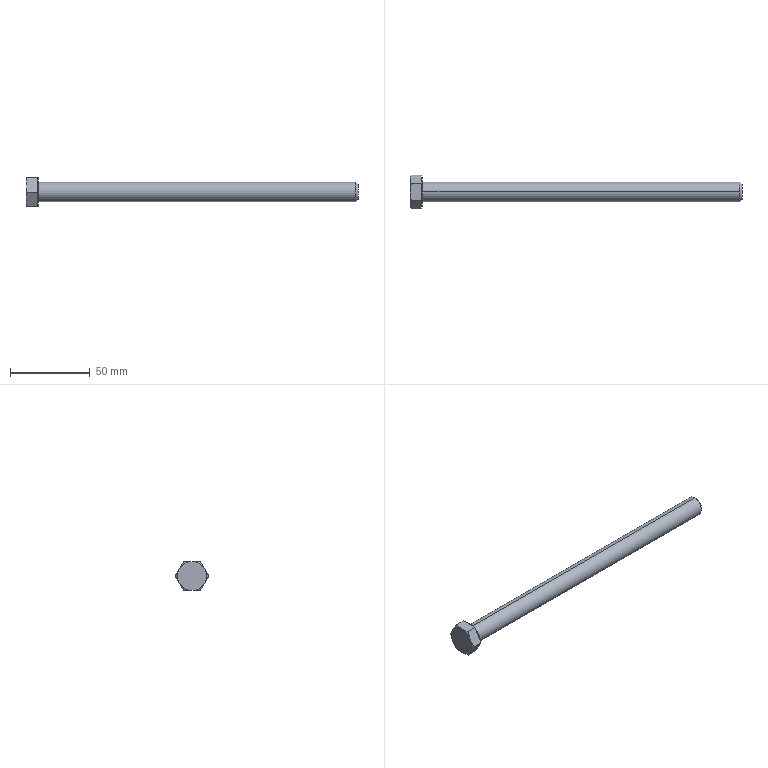Part | SolidWorks | features BaseBody 1 | 1 solid | 35 faces | box 207.5 x 20.785 x 18 mm | volume 24671 mm3 | plane 15 | cone 14 | cylinder 4 | torus 2 | commonest cylinder face diameters 12 x2 18 x2
STEP:
#1=CARTESIAN_POINT('',(8.1,0.,6.));
#2=VERTEX_POINT('',#1);
#3=CARTESIAN_POINT('',(7.5,0.,6.6));
#4=VERTEX_POINT('',#3);
#5=CARTESIAN_POINT('',(8.1,0.,6.6));
#6=DIRECTION('',(0.,1.,0.));
#7=DIRECTION('',(0.,0.,1.));
#8=AXIS2_PLACEMENT_3D('',#5,#6,#7);
#9=CIRCLE('',#8,0.6);
#10=EDGE_CURVE('',#2,#4,#9,.T.);
#11=ORIENTED_EDGE('',*,*,#10,.F.);
#12=CARTESIAN_POINT('',(8.1,0.,-6.));
#13=VERTEX_POINT('',#12);
#14=CARTESIAN_POINT('',(8.1,0.,0.));
#15=DIRECTION('',(1.,0.,0.));
#16=DIRECTION('',(0.,0.,-1.));
#17=AXIS2_PLACEMENT_3D('',#14,#15,#16);
#18=CIRCLE('',#17,6.);
#19=EDGE_CURVE('',#13,#2,#18,.T.);
#20=ORIENTED_EDGE('',*,*,#19,.F.);
#21=CARTESIAN_POINT('',(7.5,0.,-6.6));
#22=VERTEX_POINT('',#21);
#23=CARTESIAN_POINT('',(8.1,0.,-6.6));
#24=DIRECTION('',(0.,-1.,0.));
#25=DIRECTION('',(0.,0.,-1.));
#26=AXIS2_PLACEMENT_3D('',#23,#24,#25);
#27=CIRCLE('',#26,0.6);
#28=EDGE_CURVE('',#13,#22,#27,.T.);
#29=ORIENTED_EDGE('',*,*,#28,.T.);
#30=CARTESIAN_POINT('',(7.5,0.,0.));
#31=DIRECTION('',(-1.,0.,0.));
#32=DIRECTION('',(0.,0.,-1.));
#33=AXIS2_PLACEMENT_3D('',#30,#31,#32);
#34=CIRCLE('',#33,6.6);
#35=EDGE_CURVE('',#4,#22,#34,.T.);
#36=ORIENTED_EDGE('',*,*,#35,.F.);
#37=EDGE_LOOP('',(#11,#20,#29,#36));
#38=FACE_OUTER_BOUND('',#37,.T.);
#39=CARTESIAN_POINT('',(8.1,0.,0.));
#40=DIRECTION('',(1.,0.,0.));
#41=DIRECTION('',(0.,0.,-1.));
#42=AXIS2_PLACEMENT_3D('',#39,#40,#41);
#43=TOROIDAL_SURFACE('',#42,6.6,0.6);
#44=ADVANCED_FACE('',(#38),#43,.F.);
#45=CARTESIAN_POINT('',(207.5,0.,-4.6));
#46=VERTEX_POINT('',#45);
#47=CARTESIAN_POINT('',(206.1,0.,-6.));
#48=VERTEX_POINT('',#47);
#49=CARTESIAN_POINT('',(206.1,0.,-6.));
#50=DIRECTION('',(-0.7071,0.,-0.7071));
#51=VECTOR('',#50,1000.);
#52=LINE('',#49,#51);
#53=EDGE_CURVE('',#46,#48,#52,.T.);
#54=ORIENTED_EDGE('',*,*,#53,.F.);
#55=CARTESIAN_POINT('',(207.5,0.,4.6));
#56=VERTEX_POINT('',#55);
#57=CARTESIAN_POINT('',(207.5,0.,0.));
#58=DIRECTION('',(1.,0.,0.));
#59=DIRECTION('',(0.,0.,1.));
#60=AXIS2_PLACEMENT_3D('',#57,#58,#59);
#61=CIRCLE('',#60,4.6);
#62=EDGE_CURVE('',#56,#46,#61,.T.);
#63=ORIENTED_EDGE('',*,*,#62,.F.);
#64=CARTESIAN_POINT('',(206.1,0.,6.));
#65=VERTEX_POINT('',#64);
#66=CARTESIAN_POINT('',(206.1,0.,6.));
#67=DIRECTION('',(-0.7071,0.,0.7071));
#68=VECTOR('',#67,1000.);
#69=LINE('',#66,#68);
#70=EDGE_CURVE('',#56,#65,#69,.T.);
#71=ORIENTED_EDGE('',*,*,#70,.T.);
#72=CARTESIAN_POINT('',(206.1,0.,0.));
#73=DIRECTION('',(-1.,0.,0.));
#74=DIRECTION('',(0.,0.,1.));
#75=AXIS2_PLACEMENT_3D('',#72,#73,#74);
#76=CIRCLE('',#75,6.);
#77=EDGE_CURVE('',#48,#65,#76,.T.);
#78=ORIENTED_EDGE('',*,*,#77,.F.);
#79=EDGE_LOOP('',(#54,#63,#71,#78));
#80=FACE_OUTER_BOUND('',#79,.T.);
#81=CARTESIAN_POINT('',(206.1,0.,0.));
#82=DIRECTION('',(-1.,0.,0.));
#83=DIRECTION('',(0.,0.,1.));
#84=AXIS2_PLACEMENT_3D('',#81,#82,#83);
#85=CONICAL_SURFACE('',#84,6.,0.7854);
#86=ADVANCED_FACE('',(#80),#85,.T.);
#87=CARTESIAN_POINT('',(7.5,0.,0.));
#88=DIRECTION('',(-1.,0.,0.));
#89=DIRECTION('',(0.,0.,-1.));
#90=AXIS2_PLACEMENT_3D('',#87,#88,#89);
#91=CIRCLE('',#90,6.6);
#92=EDGE_CURVE('',#22,#4,#91,.T.);
#93=ORIENTED_EDGE('',*,*,#92,.T.);
#94=ORIENTED_EDGE('',*,*,#35,.T.);
#95=EDGE_LOOP('',(#93,#94));
#96=FACE_BOUND('',#95,.T.);
#97=CARTESIAN_POINT('',(7.5,0.,9.));
#98=VERTEX_POINT('',#97);
#99=CARTESIAN_POINT('',(7.5,0.,-9.));
#100=VERTEX_POINT('',#99);
#101=CARTESIAN_POINT('',(7.5,0.,0.));
#102=DIRECTION('',(1.,0.,0.));
#103=DIRECTION('',(0.,0.,-1.));
#104=AXIS2_PLACEMENT_3D('',#101,#102,#103);
#105=CIRCLE('',#104,9.);
#106=EDGE_CURVE('',#98,#100,#105,.T.);
#107=ORIENTED_EDGE('',*,*,#106,.T.);
#108=CARTESIAN_POINT('',(7.5,0.,0.));
#109=DIRECTION('',(1.,0.,0.));
#110=DIRECTION('',(0.,0.,-1.));
#111=AXIS2_PLACEMENT_3D('',#108,#109,#110);
#112=CIRCLE('',#111,9.);
#113=EDGE_CURVE('',#100,#98,#112,.T.);
#114=ORIENTED_EDGE('',*,*,#113,.T.);
#115=EDGE_LOOP('',(#107,#114));
#116=FACE_OUTER_BOUND('',#115,.T.);
#117=CARTESIAN_POINT('',(7.5,10.392,0.));
#118=DIRECTION('',(1.,0.,0.));
#119=DIRECTION('',(0.,1.,0.));
#120=AXIS2_PLACEMENT_3D('',#117,#118,#119);
#121=PLANE('',#120);
#122=ADVANCED_FACE('',(#96,#116),#121,.T.);
#123=CARTESIAN_POINT('',(0.,0.,-6.));
#124=DIRECTION('',(-1.,0.,0.));
#125=VECTOR('',#124,1000.);
#126=LINE('',#123,#125);
#127=EDGE_CURVE('',#48,#13,#126,.T.);
#128=ORIENTED_EDGE('',*,*,#127,.F.);
#129=ORIENTED_EDGE('',*,*,#77,.T.);
#130=CARTESIAN_POINT('',(0.,0.,6.));
#131=DIRECTION('',(-1.,0.,0.));
#132=VECTOR('',#131,1000.);
#133=LINE('',#130,#132);
#134=EDGE_CURVE('',#65,#2,#133,.T.);
#135=ORIENTED_EDGE('',*,*,#134,.T.);
#136=CARTESIAN_POINT('',(8.1,0.,0.));
#137=DIRECTION('',(1.,0.,0.));
#138=DIRECTION('',(0.,0.,-1.));
#139=AXIS2_PLACEMENT_3D('',#136,#137,#138);
#140=CIRCLE('',#139,6.);
#141=EDGE_CURVE('',#2,#13,#140,.T.);
#142=ORIENTED_EDGE('',*,*,#141,.T.);
#143=EDGE_LOOP('',(#128,#129,#135,#142));
#144=FACE_OUTER_BOUND('',#143,.T.);
#145=CARTESIAN_POINT('',(0.,0.,0.));
#146=DIRECTION('',(-1.,0.,0.));
#147=DIRECTION('',(0.,0.,1.));
#148=AXIS2_PLACEMENT_3D('',#145,#146,#147);
#149=CYLINDRICAL_SURFACE('',#148,6.);
#150=ADVANCED_FACE('',(#144),#149,.T.);
#151=ORIENTED_EDGE('',*,*,#62,.T.);
#152=CARTESIAN_POINT('',(207.5,0.,0.));
#153=DIRECTION('',(1.,0.,0.));
#154=DIRECTION('',(0.,0.,1.));
#155=AXIS2_PLACEMENT_3D('',#152,#153,#154);
#156=CIRCLE('',#155,4.6);
#157=EDGE_CURVE('',#46,#56,#156,.T.);
#158=ORIENTED_EDGE('',*,*,#157,.T.);
#159=EDGE_LOOP('',(#151,#158));
#160=FACE_OUTER_BOUND('',#159,.T.);
#161=CARTESIAN_POINT('',(207.5,0.,0.));
#162=DIRECTION('',(-1.,0.,0.));
#163=DIRECTION('',(0.,0.,1.));
#164=AXIS2_PLACEMENT_3D('',#161,#162,#163);
#165=PLANE('',#164);
#166=ADVANCED_FACE('',(#160),#165,.F.);
#167=CARTESIAN_POINT('',(6.9,4.448,9.));
#168=VERTEX_POINT('',#167);
#169=CARTESIAN_POINT('',(6.9,0.,9.));
#170=VERTEX_POINT('',#169);
#171=CARTESIAN_POINT('',(6.9,5.196,9.));
#172=DIRECTION('',(0.,-1.,0.));
#173=VECTOR('',#172,1000.);
#174=LINE('',#171,#173);
#175=EDGE_CURVE('',#168,#170,#174,.T.);
#176=ORIENTED_EDGE('',*,*,#175,.T.);
#177=CARTESIAN_POINT('',(6.9,7.794,4.5));
#178=VERTEX_POINT('',#177);
#179=CARTESIAN_POINT('',(6.9,0.,0.));
#180=DIRECTION('',(-1.,0.,0.));
#181=DIRECTION('',(0.,0.,1.));
#182=AXIS2_PLACEMENT_3D('',#179,#180,#181);
#183=CIRCLE('',#182,9.);
#184=EDGE_CURVE('',#170,#178,#183,.T.);
#185=ORIENTED_EDGE('',*,*,#184,.T.);
#186=CARTESIAN_POINT('',(6.9,5.57,8.352));
#187=VERTEX_POINT('',#186);
#188=CARTESIAN_POINT('',(6.9,10.392,0.));
#189=DIRECTION('',(0.,-0.5,0.866));
#190=VECTOR('',#189,1000.);
#191=LINE('',#188,#190);
#192=EDGE_CURVE('',#178,#187,#191,.T.);
#193=ORIENTED_EDGE('',*,*,#192,.T.);
#194=CARTESIAN_POINT('',(6.9,0.,0.));
#195=DIRECTION('',(-1.,0.,0.));
#196=DIRECTION('',(0.,0.,-1.));
#197=AXIS2_PLACEMENT_3D('',#194,#195,#196);
#198=CIRCLE('',#197,10.039);
#199=EDGE_CURVE('',#168,#187,#198,.T.);
#200=ORIENTED_EDGE('',*,*,#199,.F.);
#201=EDGE_LOOP('',(#176,#185,#193,#200));
#202=FACE_OUTER_BOUND('',#201,.T.);
#203=CARTESIAN_POINT('',(6.9,9.,0.));
#204=DIRECTION('',(1.,0.,0.));
#205=DIRECTION('',(0.,1.,0.));
#206=AXIS2_PLACEMENT_3D('',#203,#204,#205);
#207=PLANE('',#206);
#208=ADVANCED_FACE('',(#202),#207,.T.);
#209=CARTESIAN_POINT('',(6.9,0.,-9.));
#210=VERTEX_POINT('',#209);
#211=CARTESIAN_POINT('',(0.,0.,-9.));
#212=DIRECTION('',(-1.,0.,0.));
#213=VECTOR('',#212,1000.);
#214=LINE('',#211,#213);
#215=EDGE_CURVE('',#100,#210,#214,.T.);
#216=ORIENTED_EDGE('',*,*,#215,.F.);
#217=ORIENTED_EDGE('',*,*,#106,.F.);
#218=CARTESIAN_POINT('',(0.,0.,9.));
#219=DIRECTION('',(-1.,0.,0.));
#220=VECTOR('',#219,1000.);
#221=LINE('',#218,#220);
#222=EDGE_CURVE('',#98,#170,#221,.T.);
#223=ORIENTED_EDGE('',*,*,#222,.T.);
#224=CARTESIAN_POINT('',(6.9,-7.794,4.5));
#225=VERTEX_POINT('',#224);
#226=CARTESIAN_POINT('',(6.9,0.,0.));
#227=DIRECTION('',(-1.,0.,0.));
#228=DIRECTION('',(0.,0.,1.));
#229=AXIS2_PLACEMENT_3D('',#226,#227,#228);
#230=CIRCLE('',#229,9.);
#231=EDGE_CURVE('',#225,#170,#230,.T.);
#232=ORIENTED_EDGE('',*,*,#231,.F.);
#233=CARTESIAN_POINT('',(6.9,-7.794,-4.5));
#234=VERTEX_POINT('',#233);
#235=CARTESIAN_POINT('',(6.9,0.,0.));
#236=DIRECTION('',(-1.,0.,0.));
#237=DIRECTION('',(0.,0.,1.));
#238=AXIS2_PLACEMENT_3D('',#235,#236,#237);
#239=CIRCLE('',#238,9.);
#240=EDGE_CURVE('',#234,#225,#239,.T.);
#241=ORIENTED_EDGE('',*,*,#240,.F.);
#242=CARTESIAN_POINT('',(6.9,0.,0.));
#243=DIRECTION('',(-1.,0.,0.));
#244=DIRECTION('',(0.,0.,1.));
#245=AXIS2_PLACEMENT_3D('',#242,#243,#244);
#246=CIRCLE('',#245,9.);
#247=EDGE_CURVE('',#210,#234,#246,.T.);
#248=ORIENTED_EDGE('',*,*,#247,.F.);
#249=EDGE_LOOP('',(#216,#217,#223,#232,#241,#248));
#250=FACE_OUTER_BOUND('',#249,.T.);
#251=CARTESIAN_POINT('',(0.,0.,0.));
#252=DIRECTION('',(-1.,0.,0.));
#253=DIRECTION('',(0.,0.,1.));
#254=AXIS2_PLACEMENT_3D('',#251,#252,#253);
#255=CYLINDRICAL_SURFACE('',#254,9.);
#256=ADVANCED_FACE('',(#250),#255,.T.);
#257=CARTESIAN_POINT('',(6.9,5.57,-8.352));
#258=VERTEX_POINT('',#257);
#259=CARTESIAN_POINT('',(6.9,7.794,-4.5));
#260=VERTEX_POINT('',#259);
#261=CARTESIAN_POINT('',(6.9,5.196,-9.));
#262=DIRECTION('',(0.,0.5,0.866));
#263=VECTOR('',#262,1000.);
#264=LINE('',#261,#263);
#265=EDGE_CURVE('',#258,#260,#264,.T.);
#266=ORIENTED_EDGE('',*,*,#265,.T.);
#267=CARTESIAN_POINT('',(6.9,0.,0.));
#268=DIRECTION('',(-1.,0.,0.));
#269=DIRECTION('',(0.,0.,1.));
#270=AXIS2_PLACEMENT_3D('',#267,#268,#269);
#271=CIRCLE('',#270,9.);
#272=EDGE_CURVE('',#260,#210,#271,.T.);
#273=ORIENTED_EDGE('',*,*,#272,.T.);
#274=CARTESIAN_POINT('',(6.9,4.448,-9.));
#275=VERTEX_POINT('',#274);
#276=CARTESIAN_POINT('',(6.9,5.196,-9.));
#277=DIRECTION('',(0.,1.,0.));
#278=VECTOR('',#277,1000.);
#279=LINE('',#276,#278);
#280=EDGE_CURVE('',#210,#275,#279,.T.);
#281=ORIENTED_EDGE('',*,*,#280,.T.);
#282=CARTESIAN_POINT('',(6.9,0.,0.));
#283=DIRECTION('',(-1.,0.,0.));
#284=DIRECTION('',(0.,0.,-1.));
#285=AXIS2_PLACEMENT_3D('',#282,#283,#284);
#286=CIRCLE('',#285,10.039);
#287=EDGE_CURVE('',#258,#275,#286,.T.);
#288=ORIENTED_EDGE('',*,*,#287,.F.);
#289=EDGE_LOOP('',(#266,#273,#281,#288));
#290=FACE_OUTER_BOUND('',#289,.T.);
#291=CARTESIAN_POINT('',(6.9,9.,0.));
#292=DIRECTION('',(1.,0.,0.));
#293=DIRECTION('',(0.,1.,0.));
#294=AXIS2_PLACEMENT_3D('',#291,#292,#293);
#295=PLANE('',#294);
#296=ADVANCED_FACE('',(#290),#295,.T.);
#297=CARTESIAN_POINT('',(6.9,-5.57,-8.352));
#298=VERTEX_POINT('',#297);
#299=CARTESIAN_POINT('',(6.9,-5.196,-9.));
#300=DIRECTION('',(0.,0.5,-0.866));
#301=VECTOR('',#300,1000.);
#302=LINE('',#299,#301);
#303=EDGE_CURVE('',#234,#298,#302,.T.);
#304=ORIENTED_EDGE('',*,*,#303,.T.);
#305=CARTESIAN_POINT('',(6.9,-4.448,-9.));
#306=VERTEX_POINT('',#305);
#307=CARTESIAN_POINT('',(6.9,0.,0.));
#308=DIRECTION('',(-1.,0.,0.));
#309=DIRECTION('',(0.,0.,-1.));
#310=AXIS2_PLACEMENT_3D('',#307,#308,#309);
#311=CIRCLE('',#310,10.039);
#312=EDGE_CURVE('',#306,#298,#311,.T.);
#313=ORIENTED_EDGE('',*,*,#312,.F.);
#314=CARTESIAN_POINT('',(6.9,5.196,-9.));
#315=DIRECTION('',(0.,1.,0.));
#316=VECTOR('',#315,1000.);
#317=LINE('',#314,#316);
#318=EDGE_CURVE('',#306,#210,#317,.T.);
#319=ORIENTED_EDGE('',*,*,#318,.T.);
#320=ORIENTED_EDGE('',*,*,#247,.T.);
#321=EDGE_LOOP('',(#304,#313,#319,#320));
#322=FACE_OUTER_BOUND('',#321,.T.);
#323=CARTESIAN_POINT('',(6.9,9.,0.));
#324=DIRECTION('',(1.,0.,0.));
#325=DIRECTION('',(0.,1.,0.));
#326=AXIS2_PLACEMENT_3D('',#323,#324,#325);
#327=PLANE('',#326);
#328=ADVANCED_FACE('',(#322),#327,.T.);
#329=CARTESIAN_POINT('',(6.9,-10.018,0.6478));
#330=VERTEX_POINT('',#329);
#331=CARTESIAN_POINT('',(6.9,-10.392,0.));
#332=DIRECTION('',(0.,-0.5,-0.866));
#333=VECTOR('',#332,1000.);
#334=LINE('',#331,#333);
#335=EDGE_CURVE('',#225,#330,#334,.T.);
#336=ORIENTED_EDGE('',*,*,#335,.T.);
#337=CARTESIAN_POINT('',(6.9,-10.018,-0.6478));
#338=VERTEX_POINT('',#337);
#339=CARTESIAN_POINT('',(6.9,0.,0.));
#340=DIRECTION('',(-1.,0.,0.));
#341=DIRECTION('',(0.,0.,-1.));
#342=AXIS2_PLACEMENT_3D('',#339,#340,#341);
#343=CIRCLE('',#342,10.039);
#344=EDGE_CURVE('',#338,#330,#343,.T.);
#345=ORIENTED_EDGE('',*,*,#344,.F.);
#346=CARTESIAN_POINT('',(6.9,-5.196,-9.));
#347=DIRECTION('',(0.,0.5,-0.866));
#348=VECTOR('',#347,1000.);
#349=LINE('',#346,#348);
#350=EDGE_CURVE('',#338,#234,#349,.T.);
#351=ORIENTED_EDGE('',*,*,#350,.T.);
#352=ORIENTED_EDGE('',*,*,#240,.T.);
#353=EDGE_LOOP('',(#336,#345,#351,#352));
#354=FACE_OUTER_BOUND('',#353,.T.);
#355=CARTESIAN_POINT('',(6.9,9.,0.));
#356=DIRECTION('',(1.,0.,0.));
#357=DIRECTION('',(0.,1.,0.));
#358=AXIS2_PLACEMENT_3D('',#355,#356,#357);
#359=PLANE('',#358);
#360=ADVANCED_FACE('',(#354),#359,.T.);
#361=CARTESIAN_POINT('',(6.9,10.018,0.6478));
#362=VERTEX_POINT('',#361);
#363=CARTESIAN_POINT('',(6.9,10.392,0.));
#364=DIRECTION('',(0.,-0.5,0.866));
#365=VECTOR('',#364,1000.);
#366=LINE('',#363,#365);
#367=EDGE_CURVE('',#362,#178,#366,.T.);
#368=ORIENTED_EDGE('',*,*,#367,.T.);
#369=CARTESIAN_POINT('',(6.9,0.,0.));
#370=DIRECTION('',(-1.,0.,0.));
#371=DIRECTION('',(0.,0.,1.));
#372=AXIS2_PLACEMENT_3D('',#369,#370,#371);
#373=CIRCLE('',#372,9.);
#374=EDGE_CURVE('',#178,#260,#373,.T.);
#375=ORIENTED_EDGE('',*,*,#374,.T.);
#376=CARTESIAN_POINT('',(6.9,10.018,-0.6478));
#377=VERTEX_POINT('',#376);
#378=CARTESIAN_POINT('',(6.9,5.196,-9.));
#379=DIRECTION('',(0.,0.5,0.866));
#380=VECTOR('',#379,1000.);
#381=LINE('',#378,#380);
#382=EDGE_CURVE('',#260,#377,#381,.T.);
#383=ORIENTED_EDGE('',*,*,#382,.T.);
#384=CARTESIAN_POINT('',(6.9,0.,0.));
#385=DIRECTION('',(-1.,0.,0.));
#386=DIRECTION('',(0.,0.,-1.));
#387=AXIS2_PLACEMENT_3D('',#384,#385,#386);
#388=CIRCLE('',#387,10.039);
#389=EDGE_CURVE('',#362,#377,#388,.T.);
#390=ORIENTED_EDGE('',*,*,#389,.F.);
#391=EDGE_LOOP('',(#368,#375,#383,#390));
#392=FACE_OUTER_BOUND('',#391,.T.);
#393=CARTESIAN_POINT('',(6.9,9.,0.));
#394=DIRECTION('',(1.,0.,0.));
#395=DIRECTION('',(0.,1.,0.));
#396=AXIS2_PLACEMENT_3D('',#393,#394,#395);
#397=PLANE('',#396);
#398=ADVANCED_FACE('',(#392),#397,.T.);
#399=CARTESIAN_POINT('',(6.9,-4.448,9.));
#400=VERTEX_POINT('',#399);
#401=CARTESIAN_POINT('',(6.9,5.196,9.));
#402=DIRECTION('',(0.,-1.,0.));
#403=VECTOR('',#402,1000.);
#404=LINE('',#401,#403);
#405=EDGE_CURVE('',#170,#400,#404,.T.);
#406=ORIENTED_EDGE('',*,*,#405,.T.);
#407=CARTESIAN_POINT('',(6.9,-5.57,8.352));
#408=VERTEX_POINT('',#407);
#409=CARTESIAN_POINT('',(6.9,0.,0.));
#410=DIRECTION('',(-1.,0.,0.));
#411=DIRECTION('',(0.,0.,-1.));
#412=AXIS2_PLACEMENT_3D('',#409,#410,#411);
#413=CIRCLE('',#412,10.039);
#414=EDGE_CURVE('',#408,#400,#413,.T.);
#415=ORIENTED_EDGE('',*,*,#414,.F.);
#416=CARTESIAN_POINT('',(6.9,-10.392,0.));
#417=DIRECTION('',(0.,-0.5,-0.866));
#418=VECTOR('',#417,1000.);
#419=LINE('',#416,#418);
#420=EDGE_CURVE('',#408,#225,#419,.T.);
#421=ORIENTED_EDGE('',*,*,#420,.T.);
#422=ORIENTED_EDGE('',*,*,#231,.T.);
#423=EDGE_LOOP('',(#406,#415,#421,#422));
#424=FACE_OUTER_BOUND('',#423,.T.);
#425=CARTESIAN_POINT('',(6.9,9.,0.));
#426=DIRECTION('',(1.,0.,0.));
#427=DIRECTION('',(0.,1.,0.));
#428=AXIS2_PLACEMENT_3D('',#425,#426,#427);
#429=PLANE('',#428);
#430=ADVANCED_FACE('',(#424),#429,.T.);
#431=CARTESIAN_POINT('',(0.,0.,-9.));
#432=VERTEX_POINT('',#431);
#433=CARTESIAN_POINT('',(0.,7.794,-4.5));
#434=VERTEX_POINT('',#433);
#435=CARTESIAN_POINT('',(0.,0.,0.));
#436=DIRECTION('',(1.,0.,0.));
#437=DIRECTION('',(0.,0.,-1.));
#438=AXIS2_PLACEMENT_3D('',#435,#436,#437);
#439=CIRCLE('',#438,9.);
#440=EDGE_CURVE('',#432,#434,#439,.T.);
#441=ORIENTED_EDGE('',*,*,#440,.F.);
#442=CARTESIAN_POINT('',(0.,-7.794,-4.5));
#443=VERTEX_POINT('',#442);
#444=CARTESIAN_POINT('',(0.,0.,0.));
#445=DIRECTION('',(1.,0.,0.));
#446=DIRECTION('',(0.,0.,-1.));
#447=AXIS2_PLACEMENT_3D('',#444,#445,#446);
#448=CIRCLE('',#447,9.);
#449=EDGE_CURVE('',#443,#432,#448,.T.);
#450=ORIENTED_EDGE('',*,*,#449,.F.);
#451=CARTESIAN_POINT('',(0.,-7.794,4.5));
#452=VERTEX_POINT('',#451);
#453=CARTESIAN_POINT('',(0.,0.,0.));
#454=DIRECTION('',(1.,0.,0.));
#455=DIRECTION('',(0.,0.,-1.));
#456=AXIS2_PLACEMENT_3D('',#453,#454,#455);
#457=CIRCLE('',#456,9.);
#458=EDGE_CURVE('',#452,#443,#457,.T.);
#459=ORIENTED_EDGE('',*,*,#458,.F.);
#460=CARTESIAN_POINT('',(0.,0.,9.));
#461=VERTEX_POINT('',#460);
#462=CARTESIAN_POINT('',(0.,0.,0.));
#463=DIRECTION('',(1.,0.,0.));
#464=DIRECTION('',(0.,0.,-1.));
#465=AXIS2_PLACEMENT_3D('',#462,#463,#464);
#466=CIRCLE('',#465,9.);
#467=EDGE_CURVE('',#461,#452,#466,.T.);
#468=ORIENTED_EDGE('',*,*,#467,.F.);
#469=CARTESIAN_POINT('',(0.,7.794,4.5));
#470=VERTEX_POINT('',#469);
#471=CARTESIAN_POINT('',(0.,0.,0.));
#472=DIRECTION('',(-1.,0.,0.));
#473=DIRECTION('',(0.,0.,1.));
#474=AXIS2_PLACEMENT_3D('',#471,#472,#473);
#475=CIRCLE('',#474,9.);
#476=EDGE_CURVE('',#461,#470,#475,.T.);
#477=ORIENTED_EDGE('',*,*,#476,.T.);
#478=CARTESIAN_POINT('',(0.,0.,0.));
#479=DIRECTION('',(1.,0.,0.));
#480=DIRECTION('',(0.,0.,-1.));
#481=AXIS2_PLACEMENT_3D('',#478,#479,#480);
#482=CIRCLE('',#481,9.);
#483=EDGE_CURVE('',#434,#470,#482,.T.);
#484=ORIENTED_EDGE('',*,*,#483,.F.);
#485=EDGE_LOOP('',(#441,#450,#459,#468,#477,#484));
#486=FACE_OUTER_BOUND('',#485,.T.);
#487=CARTESIAN_POINT('',(0.,10.392,0.));
#488=DIRECTION('',(1.,0.,0.));
#489=DIRECTION('',(0.,1.,0.));
#490=AXIS2_PLACEMENT_3D('',#487,#488,#489);
#491=PLANE('',#490);
#492=ADVANCED_FACE('',(#486),#491,.F.);
#493=CARTESIAN_POINT('',(0.8038,5.196,-9.));
#494=VERTEX_POINT('',#493);
#495=CARTESIAN_POINT('',(0.,7.794,-4.5));
#496=CARTESIAN_POINT('',(0.,7.684,-4.691));
#497=CARTESIAN_POINT('',(0.004647,7.574,-4.881));
#498=CARTESIAN_POINT('',(0.01859,7.409,-5.167));
#499=CARTESIAN_POINT('',(0.0273,7.326,-5.31));
#500=CARTESIAN_POINT('',(0.03863,7.244,-5.453));
#501=CARTESIAN_POINT('',(0.04676,7.189,-5.549));
#502=CARTESIAN_POINT('',(0.05121,7.16,-5.598));
#503=CARTESIAN_POINT('',(0.07397,7.025,-5.833));
#504=CARTESIAN_POINT('',(0.09651,6.916,-6.02));
#505=CARTESIAN_POINT('',(0.1368,6.753,-6.303));
#506=CARTESIAN_POINT('',(0.1586,6.672,-6.444));
#507=CARTESIAN_POINT('',(0.1868,6.576,-6.61));
#508=CARTESIAN_POINT('',(0.1996,6.535,-6.681));
#509=CARTESIAN_POINT('',(0.2082,6.508,-6.728));
#510=CARTESIAN_POINT('',(0.2128,6.493,-6.753));
#511=CARTESIAN_POINT('',(0.3528,6.061,-7.503));
#512=CARTESIAN_POINT('',(0.5484,5.639,-8.234));
#513=CARTESIAN_POINT('',(0.8038,5.196,-9.));
#514=B_SPLINE_CURVE_WITH_KNOTS('',3,(#495,#496,#497,#498,#499,#500,#501,#502,#503,#504,#505,#506,#507,#508,#509,#510,#511,#512,#513),.UNSPECIFIED.,.F.,.F.,(4,2,1,2,2,2,1,1,2,2,4),(0.,0.125,0.1875,0.2187,0.25,0.375,0.4375,0.4687,0.4844,0.5,1.),.UNSPECIFIED.);
#515=EDGE_CURVE('',#434,#494,#514,.T.);
#516=ORIENTED_EDGE('',*,*,#515,.T.);
#517=CARTESIAN_POINT('',(0.8038,5.196,-9.));
#518=CARTESIAN_POINT('',(0.6767,4.756,-9.));
#519=CARTESIAN_POINT('',(0.5643,4.325,-9.));
#520=CARTESIAN_POINT('',(0.418,3.687,-9.));
#521=CARTESIAN_POINT('',(0.3729,3.476,-9.));
#522=CARTESIAN_POINT('',(0.3109,3.161,-9.));
#523=CARTESIAN_POINT('',(0.2812,3.004,-9.));
#524=CARTESIAN_POINT('',(0.2491,2.821,-9.));
#525=CARTESIAN_POINT('',(0.2358,2.742,-9.));
#526=CARTESIAN_POINT('',(0.2271,2.69,-9.));
#527=CARTESIAN_POINT('',(0.2231,2.665,-9.));
#528=CARTESIAN_POINT('',(0.1827,2.417,-9.));
#529=CARTESIAN_POINT('',(0.1513,2.198,-9.));
#530=CARTESIAN_POINT('',(0.1106,1.87,-9.));
#531=CARTESIAN_POINT('',(0.09818,1.761,-9.));
#532=CARTESIAN_POINT('',(0.07546,1.543,-9.));
#533=CARTESIAN_POINT('',(0.06536,1.436,-9.));
#534=CARTESIAN_POINT('',(0.01867,0.8811,-9.));
#535=CARTESIAN_POINT('',(0.,0.4425,-9.));
#536=CARTESIAN_POINT('',(0.,0.,-9.));
#537=B_SPLINE_CURVE_WITH_KNOTS('',3,(#517,#518,#519,#520,#521,#522,#523,#524,#525,#526,#527,#528,#529,#530,#531,#532,#533,#534,#535,#536),.UNSPECIFIED.,.F.,.F.,(4,2,2,1,1,2,2,2,2,2,4),(0.,0.25,0.375,0.4375,0.4688,0.4844,0.5,0.625,0.6875,0.75,1.),.UNSPECIFIED.);
#538=EDGE_CURVE('',#494,#432,#537,.T.);
#539=ORIENTED_EDGE('',*,*,#538,.T.);
#540=ORIENTED_EDGE('',*,*,#440,.T.);
#541=EDGE_LOOP('',(#516,#539,#540));
#542=FACE_OUTER_BOUND('',#541,.T.);
#543=CARTESIAN_POINT('',(0.,0.,0.));
#544=DIRECTION('',(1.,0.,0.));
#545=DIRECTION('',(0.,0.,-1.));
#546=AXIS2_PLACEMENT_3D('',#543,#544,#545);
#547=CONICAL_SURFACE('',#546,9.,1.047);
#548=ADVANCED_FACE('',(#542),#547,.T.);
#549=CARTESIAN_POINT('',(0.8038,10.392,0.));
#550=VERTEX_POINT('',#549);
#551=CARTESIAN_POINT('',(0.,7.794,4.5));
#552=CARTESIAN_POINT('',(0.,7.905,4.309));
#553=CARTESIAN_POINT('',(0.004647,8.014,4.119));
#554=CARTESIAN_POINT('',(0.01859,8.179,3.833));
#555=CARTESIAN_POINT('',(0.0273,8.262,3.69));
#556=CARTESIAN_POINT('',(0.03863,8.345,3.547));
#557=CARTESIAN_POINT('',(0.04676,8.4,3.451));
#558=CARTESIAN_POINT('',(0.05121,8.428,3.402));
#559=CARTESIAN_POINT('',(0.07397,8.564,3.167));
#560=CARTESIAN_POINT('',(0.09651,8.672,2.979));
#561=CARTESIAN_POINT('',(0.1368,8.835,2.697));
#562=CARTESIAN_POINT('',(0.1586,8.917,2.556));
#563=CARTESIAN_POINT('',(0.1868,9.012,2.39));
#564=CARTESIAN_POINT('',(0.1996,9.053,2.319));
#565=CARTESIAN_POINT('',(0.2082,9.081,2.272));
#566=CARTESIAN_POINT('',(0.2128,9.095,2.247));
#567=CARTESIAN_POINT('',(0.3528,9.528,1.497));
#568=CARTESIAN_POINT('',(0.5484,9.95,0.7662));
#569=CARTESIAN_POINT('',(0.8038,10.392,0.));
#570=B_SPLINE_CURVE_WITH_KNOTS('',3,(#551,#552,#553,#554,#555,#556,#557,#558,#559,#560,#561,#562,#563,#564,#565,#566,#567,#568,#569),.UNSPECIFIED.,.F.,.F.,(4,2,1,2,2,2,1,1,2,2,4),(0.,0.125,0.1875,0.2188,0.25,0.375,0.4375,0.4688,0.4844,0.5,1.),.UNSPECIFIED.);
#571=EDGE_CURVE('',#470,#550,#570,.T.);
#572=ORIENTED_EDGE('',*,*,#571,.T.);
#573=CARTESIAN_POINT('',(0.8038,10.392,0.));
#574=CARTESIAN_POINT('',(0.676,10.171,-0.3836));
#575=CARTESIAN_POINT('',(0.5631,9.954,-0.7585));
#576=CARTESIAN_POINT('',(0.4163,9.634,-1.313));
#577=CARTESIAN_POINT('',(0.371,9.528,-1.497));
#578=CARTESIAN_POINT('',(0.3089,9.37,-1.771));
#579=CARTESIAN_POINT('',(0.2792,9.291,-1.908));
#580=CARTESIAN_POINT('',(0.247,9.199,-2.068));
#581=CARTESIAN_POINT('',(0.2337,9.159,-2.136));
#582=CARTESIAN_POINT('',(0.225,9.133,-2.181));
#583=CARTESIAN_POINT('',(0.2209,9.12,-2.203));
#584=CARTESIAN_POINT('',(0.181,8.997,-2.417));
#585=CARTESIAN_POINT('',(0.1499,8.888,-2.605));
#586=CARTESIAN_POINT('',(0.1097,8.725,-2.887));
#587=CARTESIAN_POINT('',(0.09738,8.671,-2.981));
#588=CARTESIAN_POINT('',(0.07489,8.563,-3.169));
#589=CARTESIAN_POINT('',(0.0649,8.51,-3.261));
#590=CARTESIAN_POINT('',(0.01854,8.233,-3.74));
#591=CARTESIAN_POINT('',(0.,8.014,-4.119));
#592=CARTESIAN_POINT('',(0.,7.794,-4.5));
#593=B_SPLINE_CURVE_WITH_KNOTS('',3,(#573,#574,#575,#576,#577,#578,#579,#580,#581,#582,#583,#584,#585,#586,#587,#588,#589,#590,#591,#592),.UNSPECIFIED.,.F.,.F.,(4,2,2,1,1,2,2,2,2,2,4),(0.,0.25,0.375,0.4375,0.4687,0.4844,0.5,0.625,0.6875,0.75,1.),.UNSPECIFIED.);
#594=EDGE_CURVE('',#550,#434,#593,.T.);
#595=ORIENTED_EDGE('',*,*,#594,.T.);
#596=ORIENTED_EDGE('',*,*,#483,.T.);
#597=EDGE_LOOP('',(#572,#595,#596));
#598=FACE_OUTER_BOUND('',#597,.T.);
#599=CARTESIAN_POINT('',(0.,0.,0.));
#600=DIRECTION('',(1.,0.,0.));
#601=DIRECTION('',(0.,0.,-1.));
#602=AXIS2_PLACEMENT_3D('',#599,#600,#601);
#603=CONICAL_SURFACE('',#602,9.,1.047);
#604=ADVANCED_FACE('',(#598),#603,.T.);
#605=CARTESIAN_POINT('',(0.8038,5.196,9.));
#606=VERTEX_POINT('',#605);
#607=CARTESIAN_POINT('',(0.,0.,9.));
#608=CARTESIAN_POINT('',(0.,0.2212,9.));
#609=CARTESIAN_POINT('',(0.004668,0.4415,9.));
#610=CARTESIAN_POINT('',(0.01867,0.7722,9.));
#611=CARTESIAN_POINT('',(0.02451,0.8824,9.));
#612=CARTESIAN_POINT('',(0.03851,1.103,9.));
#613=CARTESIAN_POINT('',(0.04685,1.216,9.));
#614=CARTESIAN_POINT('',(0.07436,1.543,9.));
#615=CARTESIAN_POINT('',(0.09708,1.761,9.));
#616=CARTESIAN_POINT('',(0.1377,2.089,9.));
#617=CARTESIAN_POINT('',(0.1597,2.253,9.));
#618=CARTESIAN_POINT('',(0.1882,2.445,9.));
#619=CARTESIAN_POINT('',(0.201,2.528,9.));
#620=CARTESIAN_POINT('',(0.2097,2.583,9.));
#621=CARTESIAN_POINT('',(0.2143,2.612,9.));
#622=CARTESIAN_POINT('',(0.3544,3.474,9.));
#623=CARTESIAN_POINT('',(0.5494,4.315,9.));
#624=CARTESIAN_POINT('',(0.8038,5.196,9.));
#625=B_SPLINE_CURVE_WITH_KNOTS('',3,(#607,#608,#609,#610,#611,#612,#613,#614,#615,#616,#617,#618,#619,#620,#621,#622,#623,#624),.UNSPECIFIED.,.F.,.F.,(4,2,2,2,2,1,1,2,2,4),(0.,0.125,0.1875,0.25,0.375,0.4375,0.4687,0.4844,0.5,1.),.UNSPECIFIED.);
#626=EDGE_CURVE('',#461,#606,#625,.T.);
#627=ORIENTED_EDGE('',*,*,#626,.T.);
#628=CARTESIAN_POINT('',(0.8038,5.196,9.));
#629=CARTESIAN_POINT('',(0.676,5.418,8.616));
#630=CARTESIAN_POINT('',(0.5631,5.634,8.241));
#631=CARTESIAN_POINT('',(0.4163,5.954,7.687));
#632=CARTESIAN_POINT('',(0.371,6.06,7.503));
#633=CARTESIAN_POINT('',(0.3089,6.219,7.229));
#634=CARTESIAN_POINT('',(0.2792,6.298,7.092));
#635=CARTESIAN_POINT('',(0.247,6.39,6.932));
#636=CARTESIAN_POINT('',(0.2337,6.429,6.864));
#637=CARTESIAN_POINT('',(0.225,6.456,6.819));
#638=CARTESIAN_POINT('',(0.2209,6.468,6.797));
#639=CARTESIAN_POINT('',(0.181,6.591,6.583));
#640=CARTESIAN_POINT('',(0.1499,6.7,6.395));
#641=CARTESIAN_POINT('',(0.1097,6.863,6.113));
#642=CARTESIAN_POINT('',(0.09738,6.917,6.019));
#643=CARTESIAN_POINT('',(0.07489,7.026,5.831));
#644=CARTESIAN_POINT('',(0.0649,7.079,5.739));
#645=CARTESIAN_POINT('',(0.01854,7.356,5.26));
#646=CARTESIAN_POINT('',(0.,7.574,4.881));
#647=CARTESIAN_POINT('',(0.,7.794,4.5));
#648=B_SPLINE_CURVE_WITH_KNOTS('',3,(#628,#629,#630,#631,#632,#633,#634,#635,#636,#637,#638,#639,#640,#641,#642,#643,#644,#645,#646,#647),.UNSPECIFIED.,.F.,.F.,(4,2,2,1,1,2,2,2,2,2,4),(0.,0.25,0.375,0.4375,0.4688,0.4844,0.5,0.625,0.6875,0.75,1.),.UNSPECIFIED.);
#649=EDGE_CURVE('',#606,#470,#648,.T.);
#650=ORIENTED_EDGE('',*,*,#649,.T.);
#651=ORIENTED_EDGE('',*,*,#476,.F.);
#652=EDGE_LOOP('',(#627,#650,#651));
#653=FACE_OUTER_BOUND('',#652,.T.);
#654=CARTESIAN_POINT('',(0.,0.,0.));
#655=DIRECTION('',(1.,0.,0.));
#656=DIRECTION('',(0.,0.,-1.));
#657=AXIS2_PLACEMENT_3D('',#654,#655,#656);
#658=CONICAL_SURFACE('',#657,9.,1.047);
#659=ADVANCED_FACE('',(#653),#658,.T.);
#660=CARTESIAN_POINT('',(0.8038,-5.196,9.));
#661=VERTEX_POINT('',#660);
#662=CARTESIAN_POINT('',(0.8038,-5.196,9.));
#663=CARTESIAN_POINT('',(0.6757,-4.752,9.));
#664=CARTESIAN_POINT('',(0.5625,-4.318,9.));
#665=CARTESIAN_POINT('',(0.4154,-3.676,9.));
#666=CARTESIAN_POINT('',(0.3702,-3.463,9.));
#667=CARTESIAN_POINT('',(0.3079,-3.146,9.));
#668=CARTESIAN_POINT('',(0.2782,-2.987,9.));
#669=CARTESIAN_POINT('',(0.2506,-2.829,9.));
#670=CARTESIAN_POINT('',(0.2327,-2.724,9.));
#671=CARTESIAN_POINT('',(0.2243,-2.673,9.));
#672=CARTESIAN_POINT('',(0.1801,-2.399,9.));
#673=CARTESIAN_POINT('',(0.1491,-2.182,9.));
#674=CARTESIAN_POINT('',(0.109,-1.856,9.));
#675=CARTESIAN_POINT('',(0.09673,-1.748,9.));
#676=CARTESIAN_POINT('',(0.07432,-1.531,9.));
#677=CARTESIAN_POINT('',(0.06434,-1.424,9.));
#678=CARTESIAN_POINT('',(0.01838,-0.8733,9.));
#679=CARTESIAN_POINT('',(0.,-0.4383,9.));
#680=CARTESIAN_POINT('',(0.,0.,9.));
#681=B_SPLINE_CURVE_WITH_KNOTS('',3,(#662,#663,#664,#665,#666,#667,#668,#669,#670,#671,#672,#673,#674,#675,#676,#677,#678,#679,#680),.UNSPECIFIED.,.F.,.F.,(4,2,2,1,2,2,2,2,2,4),(0.,0.25,0.375,0.4375,0.4688,0.5,0.625,0.6875,0.75,1.),.UNSPECIFIED.);
#682=EDGE_CURVE('',#661,#461,#681,.T.);
#683=ORIENTED_EDGE('',*,*,#682,.T.);
#684=ORIENTED_EDGE('',*,*,#467,.T.);
#685=CARTESIAN_POINT('',(0.,-7.794,4.5));
#686=CARTESIAN_POINT('',(0.,-7.684,4.691));
#687=CARTESIAN_POINT('',(0.004647,-7.574,4.881));
#688=CARTESIAN_POINT('',(0.01859,-7.409,5.167));
#689=CARTESIAN_POINT('',(0.0273,-7.326,5.31));
#690=CARTESIAN_POINT('',(0.03863,-7.244,5.453));
#691=CARTESIAN_POINT('',(0.04676,-7.189,5.549));
#692=CARTESIAN_POINT('',(0.05121,-7.16,5.598));
#693=CARTESIAN_POINT('',(0.07397,-7.025,5.833));
#694=CARTESIAN_POINT('',(0.09651,-6.916,6.02));
#695=CARTESIAN_POINT('',(0.1368,-6.753,6.303));
#696=CARTESIAN_POINT('',(0.1586,-6.672,6.444));
#697=CARTESIAN_POINT('',(0.1868,-6.576,6.61));
#698=CARTESIAN_POINT('',(0.1996,-6.535,6.681));
#699=CARTESIAN_POINT('',(0.2082,-6.508,6.728));
#700=CARTESIAN_POINT('',(0.2128,-6.493,6.753));
#701=CARTESIAN_POINT('',(0.3528,-6.061,7.503));
#702=CARTESIAN_POINT('',(0.5484,-5.639,8.234));
#703=CARTESIAN_POINT('',(0.8038,-5.196,9.));
#704=B_SPLINE_CURVE_WITH_KNOTS('',3,(#685,#686,#687,#688,#689,#690,#691,#692,#693,#694,#695,#696,#697,#698,#699,#700,#701,#702,#703),.UNSPECIFIED.,.F.,.F.,(4,2,1,2,2,2,1,1,2,2,4),(0.,0.125,0.1875,0.2187,0.25,0.375,0.4375,0.4687,0.4844,0.5,1.),.UNSPECIFIED.);
#705=EDGE_CURVE('',#452,#661,#704,.T.);
#706=ORIENTED_EDGE('',*,*,#705,.T.);
#707=EDGE_LOOP('',(#683,#684,#706));
#708=FACE_OUTER_BOUND('',#707,.T.);
#709=CARTESIAN_POINT('',(0.,0.,0.));
#710=DIRECTION('',(1.,0.,0.));
#711=DIRECTION('',(0.,0.,-1.));
#712=AXIS2_PLACEMENT_3D('',#709,#710,#711);
#713=CONICAL_SURFACE('',#712,9.,1.047);
#714=ADVANCED_FACE('',(#708),#713,.T.);
#715=CARTESIAN_POINT('',(0.8038,-10.392,0.));
#716=VERTEX_POINT('',#715);
#717=CARTESIAN_POINT('',(0.8038,-10.392,0.));
#718=CARTESIAN_POINT('',(0.676,-10.171,0.3836));
#719=CARTESIAN_POINT('',(0.5631,-9.954,0.7585));
#720=CARTESIAN_POINT('',(0.4163,-9.634,1.313));
#721=CARTESIAN_POINT('',(0.371,-9.528,1.497));
#722=CARTESIAN_POINT('',(0.3089,-9.37,1.771));
#723=CARTESIAN_POINT('',(0.2792,-9.291,1.908));
#724=CARTESIAN_POINT('',(0.247,-9.199,2.068));
#725=CARTESIAN_POINT('',(0.2337,-9.159,2.136));
#726=CARTESIAN_POINT('',(0.225,-9.133,2.181));
#727=CARTESIAN_POINT('',(0.2209,-9.12,2.203));
#728=CARTESIAN_POINT('',(0.181,-8.997,2.417));
#729=CARTESIAN_POINT('',(0.1499,-8.888,2.605));
#730=CARTESIAN_POINT('',(0.1097,-8.725,2.887));
#731=CARTESIAN_POINT('',(0.09738,-8.671,2.981));
#732=CARTESIAN_POINT('',(0.07489,-8.563,3.169));
#733=CARTESIAN_POINT('',(0.0649,-8.51,3.261));
#734=CARTESIAN_POINT('',(0.01854,-8.233,3.74));
#735=CARTESIAN_POINT('',(0.,-8.014,4.119));
#736=CARTESIAN_POINT('',(0.,-7.794,4.5));
#737=B_SPLINE_CURVE_WITH_KNOTS('',3,(#717,#718,#719,#720,#721,#722,#723,#724,#725,#726,#727,#728,#729,#730,#731,#732,#733,#734,#735,#736),.UNSPECIFIED.,.F.,.F.,(4,2,2,1,1,2,2,2,2,2,4),(0.,0.25,0.375,0.4375,0.4688,0.4844,0.5,0.625,0.6875,0.75,1.),.UNSPECIFIED.);
#738=EDGE_CURVE('',#716,#452,#737,.T.);
#739=ORIENTED_EDGE('',*,*,#738,.T.);
#740=ORIENTED_EDGE('',*,*,#458,.T.);
#741=CARTESIAN_POINT('',(0.,-7.794,-4.5));
#742=CARTESIAN_POINT('',(0.,-7.905,-4.309));
#743=CARTESIAN_POINT('',(0.004647,-8.014,-4.119));
#744=CARTESIAN_POINT('',(0.01859,-8.179,-3.833));
#745=CARTESIAN_POINT('',(0.0273,-8.262,-3.69));
#746=CARTESIAN_POINT('',(0.03863,-8.345,-3.547));
#747=CARTESIAN_POINT('',(0.04676,-8.4,-3.451));
#748=CARTESIAN_POINT('',(0.05121,-8.428,-3.402));
#749=CARTESIAN_POINT('',(0.07397,-8.564,-3.167));
#750=CARTESIAN_POINT('',(0.09651,-8.672,-2.979));
#751=CARTESIAN_POINT('',(0.1368,-8.835,-2.697));
#752=CARTESIAN_POINT('',(0.1586,-8.917,-2.556));
#753=CARTESIAN_POINT('',(0.1868,-9.012,-2.39));
#754=CARTESIAN_POINT('',(0.1996,-9.053,-2.319));
#755=CARTESIAN_POINT('',(0.2082,-9.081,-2.272));
#756=CARTESIAN_POINT('',(0.2128,-9.095,-2.247));
#757=CARTESIAN_POINT('',(0.3528,-9.528,-1.497));
#758=CARTESIAN_POINT('',(0.5484,-9.95,-0.7662));
#759=CARTESIAN_POINT('',(0.8038,-10.392,0.));
#760=B_SPLINE_CURVE_WITH_KNOTS('',3,(#741,#742,#743,#744,#745,#746,#747,#748,#749,#750,#751,#752,#753,#754,#755,#756,#757,#758,#759),.UNSPECIFIED.,.F.,.F.,(4,2,1,2,2,2,1,1,2,2,4),(0.,0.125,0.1875,0.2187,0.25,0.375,0.4375,0.4687,0.4844,0.5,1.),.UNSPECIFIED.);
#761=EDGE_CURVE('',#443,#716,#760,.T.);
#762=ORIENTED_EDGE('',*,*,#761,.T.);
#763=EDGE_LOOP('',(#739,#740,#762));
#764=FACE_OUTER_BOUND('',#763,.T.);
#765=CARTESIAN_POINT('',(0.,0.,0.));
#766=DIRECTION('',(1.,0.,0.));
#767=DIRECTION('',(0.,0.,-1.));
#768=AXIS2_PLACEMENT_3D('',#765,#766,#767);
#769=CONICAL_SURFACE('',#768,9.,1.047);
#770=ADVANCED_FACE('',(#764),#769,.T.);
#771=CARTESIAN_POINT('',(0.8038,-5.196,-9.));
#772=VERTEX_POINT('',#771);
#773=CARTESIAN_POINT('',(0.8038,-5.196,-9.));
#774=CARTESIAN_POINT('',(0.676,-5.418,-8.616));
#775=CARTESIAN_POINT('',(0.5631,-5.634,-8.241));
#776=CARTESIAN_POINT('',(0.4163,-5.954,-7.687));
#777=CARTESIAN_POINT('',(0.371,-6.06,-7.503));
#778=CARTESIAN_POINT('',(0.3089,-6.219,-7.229));
#779=CARTESIAN_POINT('',(0.2792,-6.298,-7.092));
#780=CARTESIAN_POINT('',(0.247,-6.39,-6.932));
#781=CARTESIAN_POINT('',(0.2337,-6.429,-6.864));
#782=CARTESIAN_POINT('',(0.225,-6.456,-6.819));
#783=CARTESIAN_POINT('',(0.2209,-6.468,-6.797));
#784=CARTESIAN_POINT('',(0.181,-6.591,-6.583));
#785=CARTESIAN_POINT('',(0.1499,-6.7,-6.395));
#786=CARTESIAN_POINT('',(0.1097,-6.863,-6.113));
#787=CARTESIAN_POINT('',(0.09738,-6.917,-6.019));
#788=CARTESIAN_POINT('',(0.07489,-7.026,-5.831));
#789=CARTESIAN_POINT('',(0.0649,-7.079,-5.739));
#790=CARTESIAN_POINT('',(0.01854,-7.356,-5.26));
#791=CARTESIAN_POINT('',(0.,-7.574,-4.881));
#792=CARTESIAN_POINT('',(0.,-7.794,-4.5));
#793=B_SPLINE_CURVE_WITH_KNOTS('',3,(#773,#774,#775,#776,#777,#778,#779,#780,#781,#782,#783,#784,#785,#786,#787,#788,#789,#790,#791,#792),.UNSPECIFIED.,.F.,.F.,(4,2,2,1,1,2,2,2,2,2,4),(0.,0.25,0.375,0.4375,0.4688,0.4844,0.5,0.625,0.6875,0.75,1.),.UNSPECIFIED.);
#794=EDGE_CURVE('',#772,#443,#793,.T.);
#795=ORIENTED_EDGE('',*,*,#794,.T.);
#796=ORIENTED_EDGE('',*,*,#449,.T.);
#797=CARTESIAN_POINT('',(0.,0.,-9.));
#798=CARTESIAN_POINT('',(0.,-0.2191,-9.));
#799=CARTESIAN_POINT('',(0.004596,-0.4375,-9.));
#800=CARTESIAN_POINT('',(0.01838,-0.7654,-9.));
#801=CARTESIAN_POINT('',(0.02413,-0.8748,-9.));
#802=CARTESIAN_POINT('',(0.03791,-1.094,-9.));
#803=CARTESIAN_POINT('',(0.0461,-1.206,-9.));
#804=CARTESIAN_POINT('',(0.07324,-1.531,-9.));
#805=CARTESIAN_POINT('',(0.09565,-1.748,-9.));
#806=CARTESIAN_POINT('',(0.1357,-2.073,-9.));
#807=CARTESIAN_POINT('',(0.1574,-2.236,-9.));
#808=CARTESIAN_POINT('',(0.1815,-2.4,-9.));
#809=CARTESIAN_POINT('',(0.198,-2.509,-9.));
#810=CARTESIAN_POINT('',(0.207,-2.566,-9.));
#811=CARTESIAN_POINT('',(0.3513,-3.461,-9.));
#812=CARTESIAN_POINT('',(0.5475,-4.308,-9.));
#813=CARTESIAN_POINT('',(0.8038,-5.196,-9.));
#814=B_SPLINE_CURVE_WITH_KNOTS('',3,(#797,#798,#799,#800,#801,#802,#803,#804,#805,#806,#807,#808,#809,#810,#811,#812,#813),.UNSPECIFIED.,.F.,.F.,(4,2,2,2,2,1,2,2,4),(0.,0.125,0.1875,0.25,0.375,0.4375,0.4688,0.5,1.),.UNSPECIFIED.);
#815=EDGE_CURVE('',#432,#772,#814,.T.);
#816=ORIENTED_EDGE('',*,*,#815,.T.);
#817=EDGE_LOOP('',(#795,#796,#816));
#818=FACE_OUTER_BOUND('',#817,.T.);
#819=CARTESIAN_POINT('',(0.,0.,0.));
#820=DIRECTION('',(1.,0.,0.));
#821=DIRECTION('',(0.,0.,-1.));
#822=AXIS2_PLACEMENT_3D('',#819,#820,#821);
#823=CONICAL_SURFACE('',#822,9.,1.047);
#824=ADVANCED_FACE('',(#818),#823,.T.);
#825=CARTESIAN_POINT('',(6.696,5.196,-9.));
#826=VERTEX_POINT('',#825);
#827=CARTESIAN_POINT('',(6.696,5.196,-9.));
#828=CARTESIAN_POINT('',(6.768,5.321,-8.785));
#829=CARTESIAN_POINT('',(6.836,5.445,-8.569));
#830=CARTESIAN_POINT('',(6.9,5.57,-8.352));
#831=B_SPLINE_CURVE_WITH_KNOTS('',3,(#827,#828,#829,#830),.UNSPECIFIED.,.F.,.F.,(4,4),(0.000000238,0.0007696),.UNSPECIFIED.);
#832=EDGE_CURVE('',#826,#258,#831,.T.);
#833=ORIENTED_EDGE('',*,*,#832,.T.);
#834=ORIENTED_EDGE('',*,*,#287,.T.);
#835=CARTESIAN_POINT('',(6.9,4.448,-9.));
#836=CARTESIAN_POINT('',(6.836,4.698,-9.));
#837=CARTESIAN_POINT('',(6.768,4.948,-9.));
#838=CARTESIAN_POINT('',(6.696,5.196,-9.));
#839=B_SPLINE_CURVE_WITH_KNOTS('',3,(#835,#836,#837,#838),.UNSPECIFIED.,.F.,.F.,(4,4),(0.01947,0.02025),.UNSPECIFIED.);
#840=EDGE_CURVE('',#275,#826,#839,.T.);
#841=ORIENTED_EDGE('',*,*,#840,.T.);
#842=EDGE_LOOP('',(#833,#834,#841));
#843=FACE_OUTER_BOUND('',#842,.T.);
#844=CARTESIAN_POINT('',(3.809,0.,0.));
#845=DIRECTION('',(-1.,0.,0.));
#846=DIRECTION('',(0.,0.,1.));
#847=AXIS2_PLACEMENT_3D('',#844,#845,#846);
#848=CONICAL_SURFACE('',#847,15.392,1.047);
#849=ADVANCED_FACE('',(#843),#848,.T.);
#850=CARTESIAN_POINT('',(6.696,10.392,0.));
#851=VERTEX_POINT('',#850);
#852=CARTESIAN_POINT('',(6.696,10.392,0.));
#853=CARTESIAN_POINT('',(6.768,10.268,0.2154));
#854=CARTESIAN_POINT('',(6.836,10.143,0.4314));
#855=CARTESIAN_POINT('',(6.9,10.018,0.6478));
#856=B_SPLINE_CURVE_WITH_KNOTS('',3,(#852,#853,#854,#855),.UNSPECIFIED.,.F.,.F.,(4,4),(0.000000238,0.0007696),.UNSPECIFIED.);
#857=EDGE_CURVE('',#851,#362,#856,.T.);
#858=ORIENTED_EDGE('',*,*,#857,.T.);
#859=ORIENTED_EDGE('',*,*,#389,.T.);
#860=CARTESIAN_POINT('',(6.9,10.018,-0.6478));
#861=CARTESIAN_POINT('',(6.836,10.143,-0.4313));
#862=CARTESIAN_POINT('',(6.768,10.268,-0.2154));
#863=CARTESIAN_POINT('',(6.696,10.392,0.));
#864=B_SPLINE_CURVE_WITH_KNOTS('',3,(#860,#861,#862,#863),.UNSPECIFIED.,.F.,.F.,(4,4),(0.009728,0.0105),.UNSPECIFIED.);
#865=EDGE_CURVE('',#377,#851,#864,.T.);
#866=ORIENTED_EDGE('',*,*,#865,.T.);
#867=EDGE_LOOP('',(#858,#859,#866));
#868=FACE_OUTER_BOUND('',#867,.T.);
#869=CARTESIAN_POINT('',(3.809,0.,0.));
#870=DIRECTION('',(-1.,0.,0.));
#871=DIRECTION('',(0.,0.,1.));
#872=AXIS2_PLACEMENT_3D('',#869,#870,#871);
#873=CONICAL_SURFACE('',#872,15.392,1.047);
#874=ADVANCED_FACE('',(#868),#873,.T.);
#875=CARTESIAN_POINT('',(6.696,5.196,9.));
#876=VERTEX_POINT('',#875);
#877=CARTESIAN_POINT('',(6.696,5.196,9.));
#878=CARTESIAN_POINT('',(6.768,4.948,9.));
#879=CARTESIAN_POINT('',(6.836,4.698,9.));
#880=CARTESIAN_POINT('',(6.9,4.448,9.));
#881=B_SPLINE_CURVE_WITH_KNOTS('',3,(#877,#878,#879,#880),.UNSPECIFIED.,.F.,.F.,(4,4),(0.02519,0.02597),.UNSPECIFIED.);
#882=EDGE_CURVE('',#876,#168,#881,.T.);
#883=ORIENTED_EDGE('',*,*,#882,.T.);
#884=ORIENTED_EDGE('',*,*,#199,.T.);
#885=CARTESIAN_POINT('',(6.9,5.57,8.352));
#886=CARTESIAN_POINT('',(6.836,5.445,8.569));
#887=CARTESIAN_POINT('',(6.768,5.32,8.785));
#888=CARTESIAN_POINT('',(6.696,5.196,9.));
#889=B_SPLINE_CURVE_WITH_KNOTS('',3,(#885,#886,#887,#888),.UNSPECIFIED.,.F.,.F.,(4,4),(0.009728,0.0105),.UNSPECIFIED.);
#890=EDGE_CURVE('',#187,#876,#889,.T.);
#891=ORIENTED_EDGE('',*,*,#890,.T.);
#892=EDGE_LOOP('',(#883,#884,#891));
#893=FACE_OUTER_BOUND('',#892,.T.);
#894=CARTESIAN_POINT('',(3.809,0.,0.));
#895=DIRECTION('',(-1.,0.,0.));
#896=DIRECTION('',(0.,0.,1.));
#897=AXIS2_PLACEMENT_3D('',#894,#895,#896);
#898=CONICAL_SURFACE('',#897,15.392,1.047);
#899=ADVANCED_FACE('',(#893),#898,.T.);
#900=CARTESIAN_POINT('',(6.696,-5.196,9.));
#901=VERTEX_POINT('',#900);
#902=CARTESIAN_POINT('',(6.696,-5.196,9.));
#903=CARTESIAN_POINT('',(6.768,-5.321,8.785));
#904=CARTESIAN_POINT('',(6.836,-5.445,8.569));
#905=CARTESIAN_POINT('',(6.9,-5.57,8.352));
#906=B_SPLINE_CURVE_WITH_KNOTS('',3,(#902,#903,#904,#905),.UNSPECIFIED.,.F.,.F.,(4,4),(0.000000238,0.0007696),.UNSPECIFIED.);
#907=EDGE_CURVE('',#901,#408,#906,.T.);
#908=ORIENTED_EDGE('',*,*,#907,.T.);
#909=ORIENTED_EDGE('',*,*,#414,.T.);
#910=CARTESIAN_POINT('',(6.9,-4.448,9.));
#911=CARTESIAN_POINT('',(6.836,-4.699,9.));
#912=CARTESIAN_POINT('',(6.768,-4.948,9.));
#913=CARTESIAN_POINT('',(6.696,-5.196,9.));
#914=B_SPLINE_CURVE_WITH_KNOTS('',3,(#910,#911,#912,#913),.UNSPECIFIED.,.F.,.F.,(4,4),(0.03494,0.03571),.UNSPECIFIED.);
#915=EDGE_CURVE('',#400,#901,#914,.T.);
#916=ORIENTED_EDGE('',*,*,#915,.T.);
#917=EDGE_LOOP('',(#908,#909,#916));
#918=FACE_OUTER_BOUND('',#917,.T.);
#919=CARTESIAN_POINT('',(3.809,0.,0.));
#920=DIRECTION('',(-1.,0.,0.));
#921=DIRECTION('',(0.,0.,1.));
#922=AXIS2_PLACEMENT_3D('',#919,#920,#921);
#923=CONICAL_SURFACE('',#922,15.392,1.047);
#924=ADVANCED_FACE('',(#918),#923,.T.);
#925=CARTESIAN_POINT('',(6.696,-10.392,0.));
#926=VERTEX_POINT('',#925);
#927=CARTESIAN_POINT('',(6.696,-10.392,0.));
#928=CARTESIAN_POINT('',(6.768,-10.268,-0.2154));
#929=CARTESIAN_POINT('',(6.836,-10.143,-0.4314));
#930=CARTESIAN_POINT('',(6.9,-10.018,-0.6478));
#931=B_SPLINE_CURVE_WITH_KNOTS('',3,(#927,#928,#929,#930),.UNSPECIFIED.,.F.,.F.,(4,4),(0.000000238,0.0007696),.UNSPECIFIED.);
#932=EDGE_CURVE('',#926,#338,#931,.T.);
#933=ORIENTED_EDGE('',*,*,#932,.T.);
#934=ORIENTED_EDGE('',*,*,#344,.T.);
#935=CARTESIAN_POINT('',(6.9,-10.018,0.6478));
#936=CARTESIAN_POINT('',(6.836,-10.143,0.4313));
#937=CARTESIAN_POINT('',(6.768,-10.268,0.2154));
#938=CARTESIAN_POINT('',(6.696,-10.392,0.));
#939=B_SPLINE_CURVE_WITH_KNOTS('',3,(#935,#936,#937,#938),.UNSPECIFIED.,.F.,.F.,(4,4),(0.009728,0.0105),.UNSPECIFIED.);
#940=EDGE_CURVE('',#330,#926,#939,.T.);
#941=ORIENTED_EDGE('',*,*,#940,.T.);
#942=EDGE_LOOP('',(#933,#934,#941));
#943=FACE_OUTER_BOUND('',#942,.T.);
#944=CARTESIAN_POINT('',(3.809,0.,0.));
#945=DIRECTION('',(-1.,0.,0.));
#946=DIRECTION('',(0.,0.,1.));
#947=AXIS2_PLACEMENT_3D('',#944,#945,#946);
#948=CONICAL_SURFACE('',#947,15.392,1.047);
#949=ADVANCED_FACE('',(#943),#948,.T.);
#950=CARTESIAN_POINT('',(6.696,-5.196,-9.));
#951=VERTEX_POINT('',#950);
#952=CARTESIAN_POINT('',(6.696,-5.196,-9.));
#953=CARTESIAN_POINT('',(6.768,-4.948,-9.));
#954=CARTESIAN_POINT('',(6.836,-4.699,-9.));
#955=CARTESIAN_POINT('',(6.9,-4.448,-9.));
#956=B_SPLINE_CURVE_WITH_KNOTS('',3,(#952,#953,#954,#955),.UNSPECIFIED.,.F.,.F.,(4,4),(0.00972,0.01049),.UNSPECIFIED.);
#957=EDGE_CURVE('',#951,#306,#956,.T.);
#958=ORIENTED_EDGE('',*,*,#957,.T.);
#959=ORIENTED_EDGE('',*,*,#312,.T.);
#960=CARTESIAN_POINT('',(6.9,-5.57,-8.352));
#961=CARTESIAN_POINT('',(6.836,-5.445,-8.569));
#962=CARTESIAN_POINT('',(6.768,-5.32,-8.785));
#963=CARTESIAN_POINT('',(6.696,-5.196,-9.));
#964=B_SPLINE_CURVE_WITH_KNOTS('',3,(#960,#961,#962,#963),.UNSPECIFIED.,.F.,.F.,(4,4),(0.009728,0.0105),.UNSPECIFIED.);
#965=EDGE_CURVE('',#298,#951,#964,.T.);
#966=ORIENTED_EDGE('',*,*,#965,.T.);
#967=EDGE_LOOP('',(#958,#959,#966));
#968=FACE_OUTER_BOUND('',#967,.T.);
#969=CARTESIAN_POINT('',(3.809,0.,0.));
#970=DIRECTION('',(-1.,0.,0.));
#971=DIRECTION('',(0.,0.,1.));
#972=AXIS2_PLACEMENT_3D('',#969,#970,#971);
#973=CONICAL_SURFACE('',#972,15.392,1.047);
#974=ADVANCED_FACE('',(#968),#973,.T.);
#975=ORIENTED_EDGE('',*,*,#318,.F.);
#976=ORIENTED_EDGE('',*,*,#957,.F.);
#977=CARTESIAN_POINT('',(7.5,-5.196,-9.));
#978=DIRECTION('',(-1.,0.,0.));
#979=VECTOR('',#978,1000.);
#980=LINE('',#977,#979);
#981=EDGE_CURVE('',#951,#772,#980,.T.);
#982=ORIENTED_EDGE('',*,*,#981,.T.);
#983=ORIENTED_EDGE('',*,*,#815,.F.);
#984=ORIENTED_EDGE('',*,*,#538,.F.);
#985=CARTESIAN_POINT('',(7.5,5.196,-9.));
#986=DIRECTION('',(-1.,0.,0.));
#987=VECTOR('',#986,1000.);
#988=LINE('',#985,#987);
#989=EDGE_CURVE('',#826,#494,#988,.T.);
#990=ORIENTED_EDGE('',*,*,#989,.F.);
#991=ORIENTED_EDGE('',*,*,#840,.F.);
#992=ORIENTED_EDGE('',*,*,#280,.F.);
#993=EDGE_LOOP('',(#975,#976,#982,#983,#984,#990,#991,#992));
#994=FACE_OUTER_BOUND('',#993,.T.);
#995=CARTESIAN_POINT('',(7.5,5.196,-9.));
#996=DIRECTION('',(0.,0.,1.));
#997=DIRECTION('',(1.,0.,0.));
#998=AXIS2_PLACEMENT_3D('',#995,#996,#997);
#999=PLANE('',#998);
#1000=ADVANCED_FACE('',(#994),#999,.F.);
#1001=ORIENTED_EDGE('',*,*,#350,.F.);
#1002=ORIENTED_EDGE('',*,*,#932,.F.);
#1003=CARTESIAN_POINT('',(7.5,-10.392,0.));
#1004=DIRECTION('',(-1.,0.,0.));
#1005=VECTOR('',#1004,1000.);
#1006=LINE('',#1003,#1005);
#1007=EDGE_CURVE('',#926,#716,#1006,.T.);
#1008=ORIENTED_EDGE('',*,*,#1007,.T.);
#1009=ORIENTED_EDGE('',*,*,#761,.F.);
#1010=ORIENTED_EDGE('',*,*,#794,.F.);
#1011=ORIENTED_EDGE('',*,*,#981,.F.);
#1012=ORIENTED_EDGE('',*,*,#965,.F.);
#1013=ORIENTED_EDGE('',*,*,#303,.F.);
#1014=EDGE_LOOP('',(#1001,#1002,#1008,#1009,#1010,#1011,#1012,#1013));
#1015=FACE_OUTER_BOUND('',#1014,.T.);
#1016=CARTESIAN_POINT('',(7.5,-5.196,-9.));
#1017=DIRECTION('',(0.,0.866,0.5));
#1018=DIRECTION('',(1.,0.,0.));
#1019=AXIS2_PLACEMENT_3D('',#1016,#1017,#1018);
#1020=PLANE('',#1019);
#1021=ADVANCED_FACE('',(#1015),#1020,.F.);
#1022=ORIENTED_EDGE('',*,*,#420,.F.);
#1023=ORIENTED_EDGE('',*,*,#907,.F.);
#1024=CARTESIAN_POINT('',(7.5,-5.196,9.));
#1025=DIRECTION('',(-1.,0.,0.));
#1026=VECTOR('',#1025,1000.);
#1027=LINE('',#1024,#1026);
#1028=EDGE_CURVE('',#901,#661,#1027,.T.);
#1029=ORIENTED_EDGE('',*,*,#1028,.T.);
#1030=ORIENTED_EDGE('',*,*,#705,.F.);
#1031=ORIENTED_EDGE('',*,*,#738,.F.);
#1032=ORIENTED_EDGE('',*,*,#1007,.F.);
#1033=ORIENTED_EDGE('',*,*,#940,.F.);
#1034=ORIENTED_EDGE('',*,*,#335,.F.);
#1035=EDGE_LOOP('',(#1022,#1023,#1029,#1030,#1031,#1032,#1033,#1034));
#1036=FACE_OUTER_BOUND('',#1035,.T.);
#1037=CARTESIAN_POINT('',(7.5,-10.392,0.));
#1038=DIRECTION('',(0.,0.866,-0.5));
#1039=DIRECTION('',(-1.,0.,0.));
#1040=AXIS2_PLACEMENT_3D('',#1037,#1038,#1039);
#1041=PLANE('',#1040);
#1042=ADVANCED_FACE('',(#1036),#1041,.F.);
#1043=ORIENTED_EDGE('',*,*,#175,.F.);
#1044=ORIENTED_EDGE('',*,*,#882,.F.);
#1045=CARTESIAN_POINT('',(7.5,5.196,9.));
#1046=DIRECTION('',(-1.,0.,0.));
#1047=VECTOR('',#1046,1000.);
#1048=LINE('',#1045,#1047);
#1049=EDGE_CURVE('',#876,#606,#1048,.T.);
#1050=ORIENTED_EDGE('',*,*,#1049,.T.);
#1051=ORIENTED_EDGE('',*,*,#626,.F.);
#1052=ORIENTED_EDGE('',*,*,#682,.F.);
#1053=ORIENTED_EDGE('',*,*,#1028,.F.);
#1054=ORIENTED_EDGE('',*,*,#915,.F.);
#1055=ORIENTED_EDGE('',*,*,#405,.F.);
#1056=EDGE_LOOP('',(#1043,#1044,#1050,#1051,#1052,#1053,#1054,#1055));
#1057=FACE_OUTER_BOUND('',#1056,.T.);
#1058=CARTESIAN_POINT('',(7.5,5.196,9.));
#1059=DIRECTION('',(0.,0.,-1.));
#1060=DIRECTION('',(0.,-1.,0.));
#1061=AXIS2_PLACEMENT_3D('',#1058,#1059,#1060);
#1062=PLANE('',#1061);
#1063=ADVANCED_FACE('',(#1057),#1062,.F.);
#1064=ORIENTED_EDGE('',*,*,#367,.F.);
#1065=ORIENTED_EDGE('',*,*,#857,.F.);
#1066=CARTESIAN_POINT('',(7.5,10.392,0.));
#1067=DIRECTION('',(-1.,0.,0.));
#1068=VECTOR('',#1067,1000.);
#1069=LINE('',#1066,#1068);
#1070=EDGE_CURVE('',#851,#550,#1069,.T.);
#1071=ORIENTED_EDGE('',*,*,#1070,.T.);
#1072=ORIENTED_EDGE('',*,*,#571,.F.);
#1073=ORIENTED_EDGE('',*,*,#649,.F.);
#1074=ORIENTED_EDGE('',*,*,#1049,.F.);
#1075=ORIENTED_EDGE('',*,*,#890,.F.);
#1076=ORIENTED_EDGE('',*,*,#192,.F.);
#1077=EDGE_LOOP('',(#1064,#1065,#1071,#1072,#1073,#1074,#1075,#1076));
#1078=FACE_OUTER_BOUND('',#1077,.T.);
#1079=CARTESIAN_POINT('',(7.5,10.392,0.));
#1080=DIRECTION('',(0.,-0.866,-0.5));
#1081=DIRECTION('',(0.,0.5,-0.866));
#1082=AXIS2_PLACEMENT_3D('',#1079,#1080,#1081);
#1083=PLANE('',#1082);
#1084=ADVANCED_FACE('',(#1078),#1083,.F.);
#1085=ORIENTED_EDGE('',*,*,#265,.F.);
#1086=ORIENTED_EDGE('',*,*,#832,.F.);
#1087=ORIENTED_EDGE('',*,*,#989,.T.);
#1088=ORIENTED_EDGE('',*,*,#515,.F.);
#1089=ORIENTED_EDGE('',*,*,#594,.F.);
#1090=ORIENTED_EDGE('',*,*,#1070,.F.);
#1091=ORIENTED_EDGE('',*,*,#865,.F.);
#1092=ORIENTED_EDGE('',*,*,#382,.F.);
#1093=EDGE_LOOP('',(#1085,#1086,#1087,#1088,#1089,#1090,#1091,#1092));
#1094=FACE_OUTER_BOUND('',#1093,.T.);
#1095=CARTESIAN_POINT('',(7.5,5.196,-9.));
#1096=DIRECTION('',(0.,-0.866,0.5));
#1097=DIRECTION('',(-1.,0.,0.));
#1098=AXIS2_PLACEMENT_3D('',#1095,#1096,#1097);
#1099=PLANE('',#1098);
#1100=ADVANCED_FACE('',(#1094),#1099,.F.);
#1101=ORIENTED_EDGE('',*,*,#113,.F.);
#1102=ORIENTED_EDGE('',*,*,#215,.T.);
#1103=ORIENTED_EDGE('',*,*,#272,.F.);
#1104=ORIENTED_EDGE('',*,*,#374,.F.);
#1105=ORIENTED_EDGE('',*,*,#184,.F.);
#1106=ORIENTED_EDGE('',*,*,#222,.F.);
#1107=EDGE_LOOP('',(#1101,#1102,#1103,#1104,#1105,#1106));
#1108=FACE_OUTER_BOUND('',#1107,.T.);
#1109=CARTESIAN_POINT('',(0.,0.,0.));
#1110=DIRECTION('',(-1.,0.,0.));
#1111=DIRECTION('',(0.,0.,1.));
#1112=AXIS2_PLACEMENT_3D('',#1109,#1110,#1111);
#1113=CYLINDRICAL_SURFACE('',#1112,9.);
#1114=ADVANCED_FACE('',(#1108),#1113,.T.);
#1115=CARTESIAN_POINT('',(206.1,0.,0.));
#1116=DIRECTION('',(-1.,0.,0.));
#1117=DIRECTION('',(0.,0.,1.));
#1118=AXIS2_PLACEMENT_3D('',#1115,#1116,#1117);
#1119=CIRCLE('',#1118,6.);
#1120=EDGE_CURVE('',#65,#48,#1119,.T.);
#1121=ORIENTED_EDGE('',*,*,#1120,.T.);
#1122=ORIENTED_EDGE('',*,*,#127,.T.);
#1123=ORIENTED_EDGE('',*,*,#19,.T.);
#1124=ORIENTED_EDGE('',*,*,#134,.F.);
#1125=EDGE_LOOP('',(#1121,#1122,#1123,#1124));
#1126=FACE_OUTER_BOUND('',#1125,.T.);
#1127=CARTESIAN_POINT('',(0.,0.,0.));
#1128=DIRECTION('',(-1.,0.,0.));
#1129=DIRECTION('',(0.,0.,1.));
#1130=AXIS2_PLACEMENT_3D('',#1127,#1128,#1129);
#1131=CYLINDRICAL_SURFACE('',#1130,6.);
#1132=ADVANCED_FACE('',(#1126),#1131,.T.);
#1133=ORIENTED_EDGE('',*,*,#157,.F.);
#1134=ORIENTED_EDGE('',*,*,#53,.T.);
#1135=ORIENTED_EDGE('',*,*,#1120,.F.);
#1136=ORIENTED_EDGE('',*,*,#70,.F.);
#1137=EDGE_LOOP('',(#1133,#1134,#1135,#1136));
#1138=FACE_OUTER_BOUND('',#1137,.T.);
#1139=CARTESIAN_POINT('',(206.1,0.,0.));
#1140=DIRECTION('',(-1.,0.,0.));
#1141=DIRECTION('',(0.,0.,1.));
#1142=AXIS2_PLACEMENT_3D('',#1139,#1140,#1141);
#1143=CONICAL_SURFACE('',#1142,6.,0.7854);
#1144=ADVANCED_FACE('',(#1138),#1143,.T.);
#1145=ORIENTED_EDGE('',*,*,#141,.F.);
#1146=ORIENTED_EDGE('',*,*,#10,.T.);
#1147=ORIENTED_EDGE('',*,*,#92,.F.);
#1148=ORIENTED_EDGE('',*,*,#28,.F.);
#1149=EDGE_LOOP('',(#1145,#1146,#1147,#1148));
#1150=FACE_OUTER_BOUND('',#1149,.T.);
#1151=CARTESIAN_POINT('',(8.1,0.,0.));
#1152=DIRECTION('',(1.,0.,0.));
#1153=DIRECTION('',(0.,0.,-1.));
#1154=AXIS2_PLACEMENT_3D('',#1151,#1152,#1153);
#1155=TOROIDAL_SURFACE('',#1154,6.6,0.6);
#1156=ADVANCED_FACE('',(#1150),#1155,.F.);
#1157=CLOSED_SHELL('',(#44,#86,#122,#150,#166,#208,#256,#296,#328,#360,#398,#430,#492,#548,#604,#659,#714,#770,#824,#849,#874,#899,#924,#949,#974,#1000,#1021,#1042,#1063,#1084,#1100,#1114,#1132,#1144,#1156));
#1158=MANIFOLD_SOLID_BREP('',#1157);
#1159=CARTESIAN_POINT('',(0.,0.,0.));
#1160=DIRECTION('',(0.,0.,1.));
#1161=DIRECTION('',(1.,0.,0.));
#1162=AXIS2_PLACEMENT_3D('',#1159,#1160,#1161);
#1163=(LENGTH_UNIT()NAMED_UNIT(*)SI_UNIT(.MILLI.,.METRE.));
#1164=UNCERTAINTY_MEASURE_WITH_UNIT(LENGTH_MEASURE(0.00001),#1163,'','');
#1165=(NAMED_UNIT(*)PLANE_ANGLE_UNIT()SI_UNIT($,.RADIAN.));
#1166=(NAMED_UNIT(*)SI_UNIT($,.STERADIAN.)SOLID_ANGLE_UNIT());
#1167=(GEOMETRIC_REPRESENTATION_CONTEXT(3)GLOBAL_UNCERTAINTY_ASSIGNED_CONTEXT((#1164))GLOBAL_UNIT_ASSIGNED_CONTEXT((#1163,#1165,#1166))REPRESENTATION_CONTEXT('',''));
#1168=ADVANCED_BREP_SHAPE_REPRESENTATION('',(#1158,#1162),#1167);